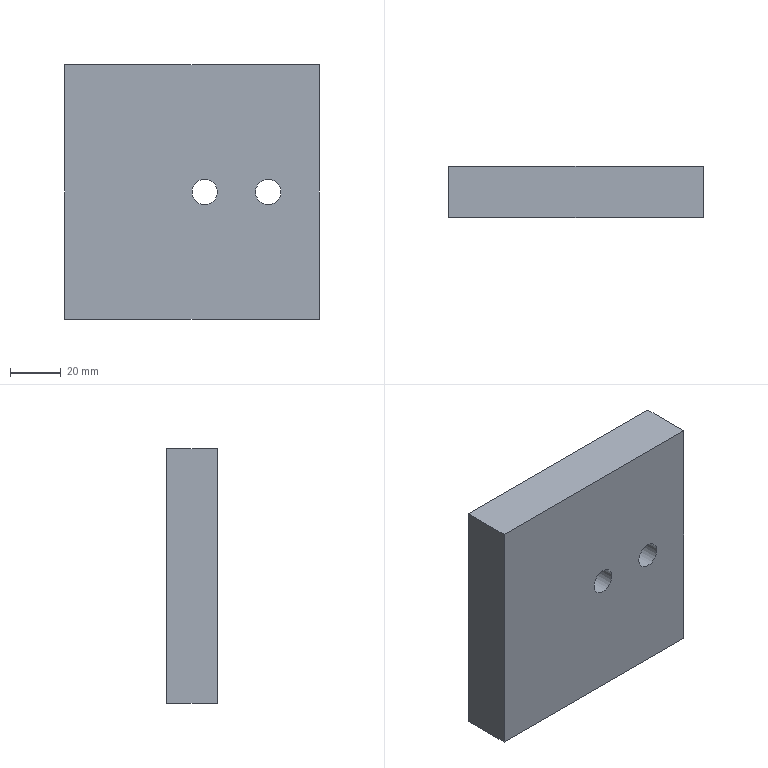Part | NX | features solid 2 | 1 solid | 8 faces | box 100 x 20 x 100 mm | volume 196858 mm3 | plane 6 | cylinder 2 | commonest cylinder face diameters 10 x2
STEP:
#1=CARTESIAN_POINT('',(-1550.,-285.,-402.5));
#2=VERTEX_POINT('',#1);
#3=CARTESIAN_POINT('',(-1550.,-265.,-402.5));
#4=VERTEX_POINT('',#3);
#5=CARTESIAN_POINT('',(-1550.,-285.,-402.5));
#6=DIRECTION('',(0.,1.,0.));
#7=VECTOR('',#6,1000.);
#8=LINE('',#5,#7);
#9=EDGE_CURVE('',#2,#4,#8,.T.);
#10=ORIENTED_EDGE('',*,*,#9,.F.);
#11=CARTESIAN_POINT('',(-1450.,-285.,-402.5));
#12=VERTEX_POINT('',#11);
#13=CARTESIAN_POINT('',(-1465.,-285.,-402.5));
#14=DIRECTION('',(-1.,0.,0.));
#15=VECTOR('',#14,1000.);
#16=LINE('',#13,#15);
#17=EDGE_CURVE('',#2,#12,#16,.F.);
#18=ORIENTED_EDGE('',*,*,#17,.T.);
#19=CARTESIAN_POINT('',(-1450.,-265.,-402.5));
#20=VERTEX_POINT('',#19);
#21=CARTESIAN_POINT('',(-1450.,-285.,-402.5));
#22=DIRECTION('',(0.,1.,0.));
#23=VECTOR('',#22,1000.);
#24=LINE('',#21,#23);
#25=EDGE_CURVE('',#12,#20,#24,.T.);
#26=ORIENTED_EDGE('',*,*,#25,.T.);
#27=CARTESIAN_POINT('',(-395.,-265.,-402.5));
#28=DIRECTION('',(1.,0.,0.));
#29=VECTOR('',#28,1000.);
#30=LINE('',#27,#29);
#31=EDGE_CURVE('',#4,#20,#30,.T.);
#32=ORIENTED_EDGE('',*,*,#31,.F.);
#33=EDGE_LOOP('',(#10,#18,#26,#32));
#34=FACE_BOUND('',#33,.T.);
#35=CARTESIAN_POINT('',(-1465.,-285.,-402.5));
#36=DIRECTION('',(0.,0.,1.));
#37=DIRECTION('',(0.,1.,0.));
#38=AXIS2_PLACEMENT_3D('',#35,#36,#37);
#39=PLANE('',#38);
#40=ADVANCED_FACE('',(#34),#39,.T.);
#41=CARTESIAN_POINT('',(-1450.,-265.,-502.5));
#42=VERTEX_POINT('',#41);
#43=CARTESIAN_POINT('',(-1450.,-265.,-907.5));
#44=DIRECTION('',(0.,0.,-1.));
#45=VECTOR('',#44,1000.);
#46=LINE('',#43,#45);
#47=EDGE_CURVE('',#20,#42,#46,.T.);
#48=ORIENTED_EDGE('',*,*,#47,.F.);
#49=ORIENTED_EDGE('',*,*,#25,.F.);
#50=CARTESIAN_POINT('',(-1450.,-285.,-502.5));
#51=VERTEX_POINT('',#50);
#52=CARTESIAN_POINT('',(-1450.,-285.,-907.5));
#53=DIRECTION('',(0.,0.,-1.));
#54=VECTOR('',#53,1000.);
#55=LINE('',#52,#54);
#56=EDGE_CURVE('',#12,#51,#55,.T.);
#57=ORIENTED_EDGE('',*,*,#56,.T.);
#58=CARTESIAN_POINT('',(-1450.,-285.,-502.5));
#59=DIRECTION('',(0.,1.,0.));
#60=VECTOR('',#59,1000.);
#61=LINE('',#58,#60);
#62=EDGE_CURVE('',#51,#42,#61,.T.);
#63=ORIENTED_EDGE('',*,*,#62,.T.);
#64=EDGE_LOOP('',(#48,#49,#57,#63));
#65=FACE_BOUND('',#64,.T.);
#66=CARTESIAN_POINT('',(-1450.,-285.,-907.5));
#67=DIRECTION('',(1.,0.,0.));
#68=DIRECTION('',(0.,1.,0.));
#69=AXIS2_PLACEMENT_3D('',#66,#67,#68);
#70=PLANE('',#69);
#71=ADVANCED_FACE('',(#65),#70,.T.);
#72=CARTESIAN_POINT('',(-1550.,-285.,-502.5));
#73=VERTEX_POINT('',#72);
#74=CARTESIAN_POINT('',(-1550.,-265.,-502.5));
#75=VERTEX_POINT('',#74);
#76=CARTESIAN_POINT('',(-1550.,-285.,-502.5));
#77=DIRECTION('',(0.,1.,0.));
#78=VECTOR('',#77,1000.);
#79=LINE('',#76,#78);
#80=EDGE_CURVE('',#73,#75,#79,.T.);
#81=ORIENTED_EDGE('',*,*,#80,.T.);
#82=CARTESIAN_POINT('',(-395.,-265.,-502.5));
#83=DIRECTION('',(-1.,0.,0.));
#84=VECTOR('',#83,1000.);
#85=LINE('',#82,#84);
#86=EDGE_CURVE('',#42,#75,#85,.T.);
#87=ORIENTED_EDGE('',*,*,#86,.F.);
#88=ORIENTED_EDGE('',*,*,#62,.F.);
#89=CARTESIAN_POINT('',(-1465.,-285.,-502.5));
#90=DIRECTION('',(-1.,0.,0.));
#91=VECTOR('',#90,1000.);
#92=LINE('',#89,#91);
#93=EDGE_CURVE('',#51,#73,#92,.T.);
#94=ORIENTED_EDGE('',*,*,#93,.T.);
#95=EDGE_LOOP('',(#81,#87,#88,#94));
#96=FACE_BOUND('',#95,.T.);
#97=CARTESIAN_POINT('',(-1465.,-285.,-502.5));
#98=DIRECTION('',(0.,0.,-1.));
#99=DIRECTION('',(0.,-1.,0.));
#100=AXIS2_PLACEMENT_3D('',#97,#98,#99);
#101=PLANE('',#100);
#102=ADVANCED_FACE('',(#96),#101,.T.);
#103=CARTESIAN_POINT('',(-1470.,-285.,-447.5));
#104=VERTEX_POINT('',#103);
#105=CARTESIAN_POINT('',(-1470.,-285.,-452.5));
#106=DIRECTION('',(0.,1.,0.));
#107=DIRECTION('',(0.,0.,1.));
#108=AXIS2_PLACEMENT_3D('',#105,#106,#107);
#109=CIRCLE('',#108,5.);
#110=EDGE_CURVE('',#104,#104,#109,.T.);
#111=ORIENTED_EDGE('',*,*,#110,.T.);
#112=EDGE_LOOP('',(#111));
#113=FACE_BOUND('',#112,.T.);
#114=CARTESIAN_POINT('',(-1495.,-285.,-447.5));
#115=VERTEX_POINT('',#114);
#116=CARTESIAN_POINT('',(-1495.,-285.,-452.5));
#117=DIRECTION('',(0.,1.,0.));
#118=DIRECTION('',(0.,0.,1.));
#119=AXIS2_PLACEMENT_3D('',#116,#117,#118);
#120=CIRCLE('',#119,5.);
#121=EDGE_CURVE('',#115,#115,#120,.T.);
#122=ORIENTED_EDGE('',*,*,#121,.T.);
#123=EDGE_LOOP('',(#122));
#124=FACE_BOUND('',#123,.T.);
#125=ORIENTED_EDGE('',*,*,#17,.F.);
#126=CARTESIAN_POINT('',(-1550.,-285.,-907.5));
#127=DIRECTION('',(0.,0.,-1.));
#128=VECTOR('',#127,1000.);
#129=LINE('',#126,#128);
#130=EDGE_CURVE('',#2,#73,#129,.T.);
#131=ORIENTED_EDGE('',*,*,#130,.T.);
#132=ORIENTED_EDGE('',*,*,#93,.F.);
#133=ORIENTED_EDGE('',*,*,#56,.F.);
#134=EDGE_LOOP('',(#125,#131,#132,#133));
#135=FACE_BOUND('',#134,.T.);
#136=CARTESIAN_POINT('',(-395.,-285.,-907.5));
#137=DIRECTION('',(0.,1.,0.));
#138=DIRECTION('',(-1.,0.,0.));
#139=AXIS2_PLACEMENT_3D('',#136,#137,#138);
#140=PLANE('',#139);
#141=ADVANCED_FACE('',(#113,#124,#135),#140,.F.);
#142=CARTESIAN_POINT('',(-1550.,-265.,-907.5));
#143=DIRECTION('',(0.,0.,-1.));
#144=VECTOR('',#143,1000.);
#145=LINE('',#142,#144);
#146=EDGE_CURVE('',#4,#75,#145,.T.);
#147=ORIENTED_EDGE('',*,*,#146,.F.);
#148=ORIENTED_EDGE('',*,*,#31,.T.);
#149=ORIENTED_EDGE('',*,*,#47,.T.);
#150=ORIENTED_EDGE('',*,*,#86,.T.);
#151=EDGE_LOOP('',(#147,#148,#149,#150));
#152=FACE_BOUND('',#151,.T.);
#153=CARTESIAN_POINT('',(-1470.,-265.,-447.5));
#154=VERTEX_POINT('',#153);
#155=CARTESIAN_POINT('',(-1470.,-265.,-452.5));
#156=DIRECTION('',(0.,1.,0.));
#157=DIRECTION('',(0.,0.,1.));
#158=AXIS2_PLACEMENT_3D('',#155,#156,#157);
#159=CIRCLE('',#158,5.);
#160=EDGE_CURVE('',#154,#154,#159,.F.);
#161=ORIENTED_EDGE('',*,*,#160,.T.);
#162=EDGE_LOOP('',(#161));
#163=FACE_BOUND('',#162,.T.);
#164=CARTESIAN_POINT('',(-1495.,-265.,-447.5));
#165=VERTEX_POINT('',#164);
#166=CARTESIAN_POINT('',(-1495.,-265.,-452.5));
#167=DIRECTION('',(0.,1.,0.));
#168=DIRECTION('',(0.,0.,1.));
#169=AXIS2_PLACEMENT_3D('',#166,#167,#168);
#170=CIRCLE('',#169,5.);
#171=EDGE_CURVE('',#165,#165,#170,.F.);
#172=ORIENTED_EDGE('',*,*,#171,.T.);
#173=EDGE_LOOP('',(#172));
#174=FACE_BOUND('',#173,.T.);
#175=CARTESIAN_POINT('',(-395.,-265.,-907.5));
#176=DIRECTION('',(0.,1.,0.));
#177=DIRECTION('',(-1.,0.,0.));
#178=AXIS2_PLACEMENT_3D('',#175,#176,#177);
#179=PLANE('',#178);
#180=ADVANCED_FACE('',(#152,#163,#174),#179,.T.);
#181=ORIENTED_EDGE('',*,*,#171,.F.);
#182=EDGE_LOOP('',(#181));
#183=FACE_BOUND('',#182,.T.);
#184=ORIENTED_EDGE('',*,*,#121,.F.);
#185=EDGE_LOOP('',(#184));
#186=FACE_BOUND('',#185,.T.);
#187=CARTESIAN_POINT('',(-1495.,-265.,-452.5));
#188=DIRECTION('',(0.,-1.,0.));
#189=DIRECTION('',(1.,0.,0.));
#190=AXIS2_PLACEMENT_3D('',#187,#188,#189);
#191=CYLINDRICAL_SURFACE('',#190,5.);
#192=ADVANCED_FACE('',(#183,#186),#191,.F.);
#193=ORIENTED_EDGE('',*,*,#160,.F.);
#194=EDGE_LOOP('',(#193));
#195=FACE_BOUND('',#194,.T.);
#196=ORIENTED_EDGE('',*,*,#110,.F.);
#197=EDGE_LOOP('',(#196));
#198=FACE_BOUND('',#197,.T.);
#199=CARTESIAN_POINT('',(-1470.,-265.,-452.5));
#200=DIRECTION('',(0.,-1.,0.));
#201=DIRECTION('',(1.,0.,0.));
#202=AXIS2_PLACEMENT_3D('',#199,#200,#201);
#203=CYLINDRICAL_SURFACE('',#202,5.);
#204=ADVANCED_FACE('',(#195,#198),#203,.F.);
#205=ORIENTED_EDGE('',*,*,#9,.T.);
#206=ORIENTED_EDGE('',*,*,#146,.T.);
#207=ORIENTED_EDGE('',*,*,#80,.F.);
#208=ORIENTED_EDGE('',*,*,#130,.F.);
#209=EDGE_LOOP('',(#205,#206,#207,#208));
#210=FACE_BOUND('',#209,.T.);
#211=CARTESIAN_POINT('',(-1550.,-285.,-907.5));
#212=DIRECTION('',(1.,0.,0.));
#213=DIRECTION('',(0.,1.,0.));
#214=AXIS2_PLACEMENT_3D('',#211,#212,#213);
#215=PLANE('',#214);
#216=ADVANCED_FACE('',(#210),#215,.F.);
#217=CLOSED_SHELL('',(#40,#71,#102,#141,#180,#192,#204,#216));
#218=MANIFOLD_SOLID_BREP('',#217);
#219=(LENGTH_UNIT()NAMED_UNIT(*)SI_UNIT(.MILLI.,.METRE.));
#220=UNCERTAINTY_MEASURE_WITH_UNIT(LENGTH_MEASURE(0.00001),#219,'','');
#221=(NAMED_UNIT(*)PLANE_ANGLE_UNIT()SI_UNIT($,.RADIAN.));
#222=(NAMED_UNIT(*)SI_UNIT($,.STERADIAN.)SOLID_ANGLE_UNIT());
#223=(GEOMETRIC_REPRESENTATION_CONTEXT(3)GLOBAL_UNCERTAINTY_ASSIGNED_CONTEXT((#220))GLOBAL_UNIT_ASSIGNED_CONTEXT((#219,#221,#222))REPRESENTATION_CONTEXT('',''));
#224=ADVANCED_BREP_SHAPE_REPRESENTATION('',(#218),#223);